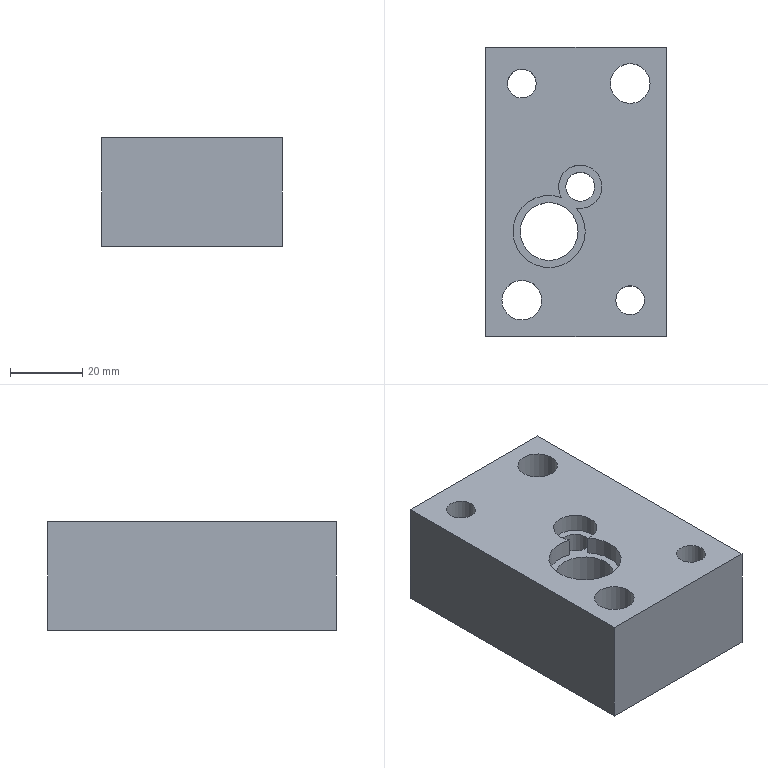Part | NX | features solid 2 | 1 solid | 19 faces | box 50 x 80 x 30 mm | volume 98920 mm3 | cylinder 10 | plane 9 | commonest cylinder face diameters 8 x3 11 x2 17 x2 12 x1 16 x1 20 x1
STEP:
#1=CARTESIAN_POINT('',(-537.829,181.45,124.));
#2=VERTEX_POINT('',#1);
#3=CARTESIAN_POINT('',(-533.829,181.45,124.));
#4=DIRECTION('',(0.,0.,-1.));
#5=DIRECTION('',(-1.,0.,0.));
#6=AXIS2_PLACEMENT_3D('',#3,#4,#5);
#7=CIRCLE('',#6,4.);
#8=EDGE_CURVE('',#2,#2,#7,.F.);
#9=ORIENTED_EDGE('',*,*,#8,.T.);
#10=EDGE_LOOP('',(#9));
#11=FACE_BOUND('',#10,.T.);
#12=CARTESIAN_POINT('',(-528.5,210.,124.));
#13=VERTEX_POINT('',#12);
#14=CARTESIAN_POINT('',(-520.,210.,124.));
#15=DIRECTION('',(0.,0.,-1.));
#16=DIRECTION('',(-1.,0.,0.));
#17=AXIS2_PLACEMENT_3D('',#14,#15,#16);
#18=CIRCLE('',#17,8.5);
#19=EDGE_CURVE('',#13,#13,#18,.T.);
#20=ORIENTED_EDGE('',*,*,#19,.F.);
#21=EDGE_LOOP('',(#20));
#22=FACE_BOUND('',#21,.T.);
#23=CARTESIAN_POINT('',(-558.5,150.,124.));
#24=VERTEX_POINT('',#23);
#25=CARTESIAN_POINT('',(-550.,150.,124.));
#26=DIRECTION('',(0.,0.,-1.));
#27=DIRECTION('',(-1.,0.,0.));
#28=AXIS2_PLACEMENT_3D('',#25,#26,#27);
#29=CIRCLE('',#28,8.5);
#30=EDGE_CURVE('',#24,#24,#29,.T.);
#31=ORIENTED_EDGE('',*,*,#30,.F.);
#32=EDGE_LOOP('',(#31));
#33=FACE_BOUND('',#32,.T.);
#34=CARTESIAN_POINT('',(-554.,210.,124.));
#35=VERTEX_POINT('',#34);
#36=CARTESIAN_POINT('',(-550.,210.,124.));
#37=DIRECTION('',(0.,0.,-1.));
#38=DIRECTION('',(-1.,0.,0.));
#39=AXIS2_PLACEMENT_3D('',#36,#37,#38);
#40=CIRCLE('',#39,4.);
#41=EDGE_CURVE('',#35,#35,#40,.T.);
#42=ORIENTED_EDGE('',*,*,#41,.F.);
#43=EDGE_LOOP('',(#42));
#44=FACE_BOUND('',#43,.T.);
#45=CARTESIAN_POINT('',(-524.,150.,124.));
#46=VERTEX_POINT('',#45);
#47=CARTESIAN_POINT('',(-520.,150.,124.));
#48=DIRECTION('',(0.,0.,-1.));
#49=DIRECTION('',(-1.,0.,0.));
#50=AXIS2_PLACEMENT_3D('',#47,#48,#49);
#51=CIRCLE('',#50,4.);
#52=EDGE_CURVE('',#46,#46,#51,.T.);
#53=ORIENTED_EDGE('',*,*,#52,.F.);
#54=EDGE_LOOP('',(#53));
#55=FACE_BOUND('',#54,.T.);
#56=CARTESIAN_POINT('',(-510.,220.,124.));
#57=VERTEX_POINT('',#56);
#58=CARTESIAN_POINT('',(-560.,220.,124.));
#59=VERTEX_POINT('',#58);
#60=CARTESIAN_POINT('',(-495.,220.,124.));
#61=DIRECTION('',(-1.,0.,0.));
#62=VECTOR('',#61,1000.);
#63=LINE('',#60,#62);
#64=EDGE_CURVE('',#57,#59,#63,.T.);
#65=ORIENTED_EDGE('',*,*,#64,.F.);
#66=CARTESIAN_POINT('',(-510.,140.,124.));
#67=VERTEX_POINT('',#66);
#68=CARTESIAN_POINT('',(-510.,205.,124.));
#69=DIRECTION('',(0.,1.,0.));
#70=VECTOR('',#69,1000.);
#71=LINE('',#68,#70);
#72=EDGE_CURVE('',#67,#57,#71,.T.);
#73=ORIENTED_EDGE('',*,*,#72,.F.);
#74=CARTESIAN_POINT('',(-560.,140.,124.));
#75=VERTEX_POINT('',#74);
#76=CARTESIAN_POINT('',(-495.,140.,124.));
#77=DIRECTION('',(1.,0.,0.));
#78=VECTOR('',#77,1000.);
#79=LINE('',#76,#78);
#80=EDGE_CURVE('',#75,#67,#79,.T.);
#81=ORIENTED_EDGE('',*,*,#80,.F.);
#82=CARTESIAN_POINT('',(-560.,205.,124.));
#83=DIRECTION('',(0.,-1.,0.));
#84=VECTOR('',#83,1000.);
#85=LINE('',#82,#84);
#86=EDGE_CURVE('',#59,#75,#85,.T.);
#87=ORIENTED_EDGE('',*,*,#86,.F.);
#88=EDGE_LOOP('',(#65,#73,#81,#87));
#89=FACE_BOUND('',#88,.T.);
#90=CARTESIAN_POINT('',(-550.438,169.049,124.));
#91=VERTEX_POINT('',#90);
#92=CARTESIAN_POINT('',(-542.438,169.049,124.));
#93=DIRECTION('',(0.,0.,-1.));
#94=DIRECTION('',(-1.,0.,0.));
#95=AXIS2_PLACEMENT_3D('',#92,#93,#94);
#96=CIRCLE('',#95,8.);
#97=EDGE_CURVE('',#91,#91,#96,.F.);
#98=ORIENTED_EDGE('',*,*,#97,.T.);
#99=EDGE_LOOP('',(#98));
#100=FACE_BOUND('',#99,.T.);
#101=CARTESIAN_POINT('',(-495.,205.,124.));
#102=DIRECTION('',(0.,0.,-1.));
#103=DIRECTION('',(1.,0.,0.));
#104=AXIS2_PLACEMENT_3D('',#101,#102,#103);
#105=PLANE('',#104);
#106=ADVANCED_FACE('',(#11,#22,#33,#44,#55,#89,#100),#105,.T.);
#107=CARTESIAN_POINT('',(-510.,140.,154.));
#108=VERTEX_POINT('',#107);
#109=CARTESIAN_POINT('',(-510.,220.,154.));
#110=VERTEX_POINT('',#109);
#111=CARTESIAN_POINT('',(-510.,169.049,154.));
#112=DIRECTION('',(0.,-1.,0.));
#113=VECTOR('',#112,1000.);
#114=LINE('',#111,#113);
#115=EDGE_CURVE('',#108,#110,#114,.F.);
#116=ORIENTED_EDGE('',*,*,#115,.F.);
#117=CARTESIAN_POINT('',(-510.,140.,128.));
#118=DIRECTION('',(0.,0.,1.));
#119=VECTOR('',#118,1000.);
#120=LINE('',#117,#119);
#121=EDGE_CURVE('',#67,#108,#120,.T.);
#122=ORIENTED_EDGE('',*,*,#121,.F.);
#123=ORIENTED_EDGE('',*,*,#72,.T.);
#124=CARTESIAN_POINT('',(-510.,220.,128.));
#125=DIRECTION('',(0.,0.,1.));
#126=VECTOR('',#125,1000.);
#127=LINE('',#124,#126);
#128=EDGE_CURVE('',#57,#110,#127,.T.);
#129=ORIENTED_EDGE('',*,*,#128,.T.);
#130=EDGE_LOOP('',(#116,#122,#123,#129));
#131=FACE_BOUND('',#130,.T.);
#132=CARTESIAN_POINT('',(-510.,155.,128.));
#133=DIRECTION('',(-1.,0.,0.));
#134=DIRECTION('',(0.,0.,-1.));
#135=AXIS2_PLACEMENT_3D('',#132,#133,#134);
#136=PLANE('',#135);
#137=ADVANCED_FACE('',(#131),#136,.F.);
#138=CARTESIAN_POINT('',(-560.,220.,154.));
#139=VERTEX_POINT('',#138);
#140=CARTESIAN_POINT('',(-542.438,220.,154.));
#141=DIRECTION('',(1.,0.,0.));
#142=VECTOR('',#141,1000.);
#143=LINE('',#140,#142);
#144=EDGE_CURVE('',#110,#139,#143,.F.);
#145=ORIENTED_EDGE('',*,*,#144,.F.);
#146=ORIENTED_EDGE('',*,*,#128,.F.);
#147=ORIENTED_EDGE('',*,*,#64,.T.);
#148=CARTESIAN_POINT('',(-560.,220.,128.));
#149=DIRECTION('',(0.,0.,1.));
#150=VECTOR('',#149,1000.);
#151=LINE('',#148,#150);
#152=EDGE_CURVE('',#59,#139,#151,.T.);
#153=ORIENTED_EDGE('',*,*,#152,.T.);
#154=EDGE_LOOP('',(#145,#146,#147,#153));
#155=FACE_BOUND('',#154,.T.);
#156=CARTESIAN_POINT('',(-495.,220.,128.));
#157=DIRECTION('',(0.,-1.,0.));
#158=DIRECTION('',(0.,0.,-1.));
#159=AXIS2_PLACEMENT_3D('',#156,#157,#158);
#160=PLANE('',#159);
#161=ADVANCED_FACE('',(#155),#160,.F.);
#162=ORIENTED_EDGE('',*,*,#86,.T.);
#163=CARTESIAN_POINT('',(-560.,140.,154.));
#164=VERTEX_POINT('',#163);
#165=CARTESIAN_POINT('',(-560.,140.,128.));
#166=DIRECTION('',(0.,0.,1.));
#167=VECTOR('',#166,1000.);
#168=LINE('',#165,#167);
#169=EDGE_CURVE('',#75,#164,#168,.T.);
#170=ORIENTED_EDGE('',*,*,#169,.T.);
#171=CARTESIAN_POINT('',(-560.,169.049,154.));
#172=DIRECTION('',(0.,1.,0.));
#173=VECTOR('',#172,1000.);
#174=LINE('',#171,#173);
#175=EDGE_CURVE('',#139,#164,#174,.F.);
#176=ORIENTED_EDGE('',*,*,#175,.F.);
#177=ORIENTED_EDGE('',*,*,#152,.F.);
#178=EDGE_LOOP('',(#162,#170,#176,#177));
#179=FACE_BOUND('',#178,.T.);
#180=CARTESIAN_POINT('',(-560.,205.,128.));
#181=DIRECTION('',(1.,0.,0.));
#182=DIRECTION('',(0.,0.,1.));
#183=AXIS2_PLACEMENT_3D('',#180,#181,#182);
#184=PLANE('',#183);
#185=ADVANCED_FACE('',(#179),#184,.F.);
#186=CARTESIAN_POINT('',(-542.438,140.,154.));
#187=DIRECTION('',(-1.,0.,0.));
#188=VECTOR('',#187,1000.);
#189=LINE('',#186,#188);
#190=EDGE_CURVE('',#164,#108,#189,.F.);
#191=ORIENTED_EDGE('',*,*,#190,.F.);
#192=ORIENTED_EDGE('',*,*,#169,.F.);
#193=ORIENTED_EDGE('',*,*,#80,.T.);
#194=ORIENTED_EDGE('',*,*,#121,.T.);
#195=EDGE_LOOP('',(#191,#192,#193,#194));
#196=FACE_BOUND('',#195,.T.);
#197=CARTESIAN_POINT('',(-550.,140.,128.));
#198=DIRECTION('',(0.,1.,0.));
#199=DIRECTION('',(0.,0.,1.));
#200=AXIS2_PLACEMENT_3D('',#197,#198,#199);
#201=PLANE('',#200);
#202=ADVANCED_FACE('',(#196),#201,.F.);
#203=CARTESIAN_POINT('',(-539.024,178.448,154.));
#204=VERTEX_POINT('',#203);
#205=CARTESIAN_POINT('',(-534.825,175.533,154.));
#206=VERTEX_POINT('',#205);
#207=CARTESIAN_POINT('',(-542.438,169.049,154.));
#208=DIRECTION('',(0.,0.,1.));
#209=DIRECTION('',(1.,0.,0.));
#210=AXIS2_PLACEMENT_3D('',#207,#208,#209);
#211=CIRCLE('',#210,10.);
#212=EDGE_CURVE('',#204,#206,#211,.T.);
#213=ORIENTED_EDGE('',*,*,#212,.F.);
#214=CARTESIAN_POINT('',(-533.829,181.45,154.));
#215=DIRECTION('',(0.,0.,1.));
#216=DIRECTION('',(1.,0.,0.));
#217=AXIS2_PLACEMENT_3D('',#214,#215,#216);
#218=CIRCLE('',#217,6.);
#219=EDGE_CURVE('',#206,#204,#218,.T.);
#220=ORIENTED_EDGE('',*,*,#219,.F.);
#221=EDGE_LOOP('',(#213,#220));
#222=FACE_BOUND('',#221,.T.);
#223=CARTESIAN_POINT('',(-514.5,210.,154.));
#224=VERTEX_POINT('',#223);
#225=CARTESIAN_POINT('',(-520.,210.,154.));
#226=DIRECTION('',(0.,0.,1.));
#227=DIRECTION('',(1.,0.,0.));
#228=AXIS2_PLACEMENT_3D('',#225,#226,#227);
#229=CIRCLE('',#228,5.5);
#230=EDGE_CURVE('',#224,#224,#229,.T.);
#231=ORIENTED_EDGE('',*,*,#230,.F.);
#232=EDGE_LOOP('',(#231));
#233=FACE_BOUND('',#232,.T.);
#234=CARTESIAN_POINT('',(-544.5,150.,154.));
#235=VERTEX_POINT('',#234);
#236=CARTESIAN_POINT('',(-550.,150.,154.));
#237=DIRECTION('',(0.,0.,1.));
#238=DIRECTION('',(1.,0.,0.));
#239=AXIS2_PLACEMENT_3D('',#236,#237,#238);
#240=CIRCLE('',#239,5.5);
#241=EDGE_CURVE('',#235,#235,#240,.T.);
#242=ORIENTED_EDGE('',*,*,#241,.F.);
#243=EDGE_LOOP('',(#242));
#244=FACE_BOUND('',#243,.T.);
#245=CARTESIAN_POINT('',(-546.,210.,154.));
#246=VERTEX_POINT('',#245);
#247=CARTESIAN_POINT('',(-550.,210.,154.));
#248=DIRECTION('',(0.,0.,1.));
#249=DIRECTION('',(1.,0.,0.));
#250=AXIS2_PLACEMENT_3D('',#247,#248,#249);
#251=CIRCLE('',#250,4.);
#252=EDGE_CURVE('',#246,#246,#251,.T.);
#253=ORIENTED_EDGE('',*,*,#252,.F.);
#254=EDGE_LOOP('',(#253));
#255=FACE_BOUND('',#254,.T.);
#256=CARTESIAN_POINT('',(-516.,150.,154.));
#257=VERTEX_POINT('',#256);
#258=CARTESIAN_POINT('',(-520.,150.,154.));
#259=DIRECTION('',(0.,0.,1.));
#260=DIRECTION('',(1.,0.,0.));
#261=AXIS2_PLACEMENT_3D('',#258,#259,#260);
#262=CIRCLE('',#261,4.);
#263=EDGE_CURVE('',#257,#257,#262,.T.);
#264=ORIENTED_EDGE('',*,*,#263,.F.);
#265=EDGE_LOOP('',(#264));
#266=FACE_BOUND('',#265,.T.);
#267=ORIENTED_EDGE('',*,*,#175,.T.);
#268=ORIENTED_EDGE('',*,*,#190,.T.);
#269=ORIENTED_EDGE('',*,*,#115,.T.);
#270=ORIENTED_EDGE('',*,*,#144,.T.);
#271=EDGE_LOOP('',(#267,#268,#269,#270));
#272=FACE_BOUND('',#271,.T.);
#273=CARTESIAN_POINT('',(-542.438,169.049,154.));
#274=DIRECTION('',(0.,0.,1.));
#275=DIRECTION('',(1.,0.,0.));
#276=AXIS2_PLACEMENT_3D('',#273,#274,#275);
#277=PLANE('',#276);
#278=ADVANCED_FACE('',(#222,#233,#244,#255,#266,#272),#277,.T.);
#279=ORIENTED_EDGE('',*,*,#263,.T.);
#280=EDGE_LOOP('',(#279));
#281=FACE_BOUND('',#280,.T.);
#282=ORIENTED_EDGE('',*,*,#52,.T.);
#283=EDGE_LOOP('',(#282));
#284=FACE_BOUND('',#283,.T.);
#285=CARTESIAN_POINT('',(-520.,150.,178.));
#286=DIRECTION('',(0.,0.,1.));
#287=DIRECTION('',(-1.,0.,0.));
#288=AXIS2_PLACEMENT_3D('',#285,#286,#287);
#289=CYLINDRICAL_SURFACE('',#288,4.);
#290=ADVANCED_FACE('',(#281,#284),#289,.F.);
#291=ORIENTED_EDGE('',*,*,#252,.T.);
#292=EDGE_LOOP('',(#291));
#293=FACE_BOUND('',#292,.T.);
#294=ORIENTED_EDGE('',*,*,#41,.T.);
#295=EDGE_LOOP('',(#294));
#296=FACE_BOUND('',#295,.T.);
#297=CARTESIAN_POINT('',(-550.,210.,178.));
#298=DIRECTION('',(0.,0.,1.));
#299=DIRECTION('',(-1.,0.,0.));
#300=AXIS2_PLACEMENT_3D('',#297,#298,#299);
#301=CYLINDRICAL_SURFACE('',#300,4.);
#302=ADVANCED_FACE('',(#293,#296),#301,.F.);
#303=CARTESIAN_POINT('',(-544.5,150.,139.));
#304=VERTEX_POINT('',#303);
#305=CARTESIAN_POINT('',(-550.,150.,139.));
#306=DIRECTION('',(0.,0.,1.));
#307=DIRECTION('',(1.,0.,0.));
#308=AXIS2_PLACEMENT_3D('',#305,#306,#307);
#309=CIRCLE('',#308,5.5);
#310=EDGE_CURVE('',#304,#304,#309,.F.);
#311=ORIENTED_EDGE('',*,*,#310,.T.);
#312=EDGE_LOOP('',(#311));
#313=FACE_BOUND('',#312,.T.);
#314=ORIENTED_EDGE('',*,*,#241,.T.);
#315=EDGE_LOOP('',(#314));
#316=FACE_BOUND('',#315,.T.);
#317=CARTESIAN_POINT('',(-550.,150.,178.));
#318=DIRECTION('',(0.,0.,1.));
#319=DIRECTION('',(-1.,0.,0.));
#320=AXIS2_PLACEMENT_3D('',#317,#318,#319);
#321=CYLINDRICAL_SURFACE('',#320,5.5);
#322=ADVANCED_FACE('',(#313,#316),#321,.F.);
#323=ORIENTED_EDGE('',*,*,#310,.F.);
#324=EDGE_LOOP('',(#323));
#325=FACE_BOUND('',#324,.T.);
#326=CARTESIAN_POINT('',(-541.5,150.,139.));
#327=VERTEX_POINT('',#326);
#328=CARTESIAN_POINT('',(-550.,150.,139.));
#329=DIRECTION('',(0.,0.,1.));
#330=DIRECTION('',(1.,0.,0.));
#331=AXIS2_PLACEMENT_3D('',#328,#329,#330);
#332=CIRCLE('',#331,8.5);
#333=EDGE_CURVE('',#327,#327,#332,.F.);
#334=ORIENTED_EDGE('',*,*,#333,.T.);
#335=EDGE_LOOP('',(#334));
#336=FACE_BOUND('',#335,.T.);
#337=CARTESIAN_POINT('',(-550.,150.,139.));
#338=DIRECTION('',(0.,0.,1.));
#339=DIRECTION('',(-1.,0.,0.));
#340=AXIS2_PLACEMENT_3D('',#337,#338,#339);
#341=PLANE('',#340);
#342=ADVANCED_FACE('',(#325,#336),#341,.F.);
#343=ORIENTED_EDGE('',*,*,#333,.F.);
#344=EDGE_LOOP('',(#343));
#345=FACE_BOUND('',#344,.T.);
#346=ORIENTED_EDGE('',*,*,#30,.T.);
#347=EDGE_LOOP('',(#346));
#348=FACE_BOUND('',#347,.T.);
#349=CARTESIAN_POINT('',(-550.,150.,128.));
#350=DIRECTION('',(0.,0.,1.));
#351=DIRECTION('',(-1.,0.,0.));
#352=AXIS2_PLACEMENT_3D('',#349,#350,#351);
#353=CYLINDRICAL_SURFACE('',#352,8.5);
#354=ADVANCED_FACE('',(#345,#348),#353,.F.);
#355=CARTESIAN_POINT('',(-514.5,210.,139.));
#356=VERTEX_POINT('',#355);
#357=CARTESIAN_POINT('',(-520.,210.,139.));
#358=DIRECTION('',(0.,0.,1.));
#359=DIRECTION('',(1.,0.,0.));
#360=AXIS2_PLACEMENT_3D('',#357,#358,#359);
#361=CIRCLE('',#360,5.5);
#362=EDGE_CURVE('',#356,#356,#361,.F.);
#363=ORIENTED_EDGE('',*,*,#362,.T.);
#364=EDGE_LOOP('',(#363));
#365=FACE_BOUND('',#364,.T.);
#366=ORIENTED_EDGE('',*,*,#230,.T.);
#367=EDGE_LOOP('',(#366));
#368=FACE_BOUND('',#367,.T.);
#369=CARTESIAN_POINT('',(-520.,210.,178.));
#370=DIRECTION('',(0.,0.,1.));
#371=DIRECTION('',(-1.,0.,0.));
#372=AXIS2_PLACEMENT_3D('',#369,#370,#371);
#373=CYLINDRICAL_SURFACE('',#372,5.5);
#374=ADVANCED_FACE('',(#365,#368),#373,.F.);
#375=ORIENTED_EDGE('',*,*,#362,.F.);
#376=EDGE_LOOP('',(#375));
#377=FACE_BOUND('',#376,.T.);
#378=CARTESIAN_POINT('',(-511.5,210.,139.));
#379=VERTEX_POINT('',#378);
#380=CARTESIAN_POINT('',(-520.,210.,139.));
#381=DIRECTION('',(0.,0.,1.));
#382=DIRECTION('',(1.,0.,0.));
#383=AXIS2_PLACEMENT_3D('',#380,#381,#382);
#384=CIRCLE('',#383,8.5);
#385=EDGE_CURVE('',#379,#379,#384,.F.);
#386=ORIENTED_EDGE('',*,*,#385,.T.);
#387=EDGE_LOOP('',(#386));
#388=FACE_BOUND('',#387,.T.);
#389=CARTESIAN_POINT('',(-520.,210.,139.));
#390=DIRECTION('',(0.,0.,1.));
#391=DIRECTION('',(-1.,0.,0.));
#392=AXIS2_PLACEMENT_3D('',#389,#390,#391);
#393=PLANE('',#392);
#394=ADVANCED_FACE('',(#377,#388),#393,.F.);
#395=ORIENTED_EDGE('',*,*,#385,.F.);
#396=EDGE_LOOP('',(#395));
#397=FACE_BOUND('',#396,.T.);
#398=ORIENTED_EDGE('',*,*,#19,.T.);
#399=EDGE_LOOP('',(#398));
#400=FACE_BOUND('',#399,.T.);
#401=CARTESIAN_POINT('',(-520.,210.,128.));
#402=DIRECTION('',(0.,0.,1.));
#403=DIRECTION('',(-1.,0.,0.));
#404=AXIS2_PLACEMENT_3D('',#401,#402,#403);
#405=CYLINDRICAL_SURFACE('',#404,8.5);
#406=ADVANCED_FACE('',(#397,#400),#405,.F.);
#407=ORIENTED_EDGE('',*,*,#8,.F.);
#408=EDGE_LOOP('',(#407));
#409=FACE_BOUND('',#408,.T.);
#410=CARTESIAN_POINT('',(-529.829,181.45,149.));
#411=VERTEX_POINT('',#410);
#412=CARTESIAN_POINT('',(-533.829,181.45,149.));
#413=DIRECTION('',(0.,0.,1.));
#414=DIRECTION('',(1.,0.,0.));
#415=AXIS2_PLACEMENT_3D('',#412,#413,#414);
#416=CIRCLE('',#415,4.);
#417=EDGE_CURVE('',#411,#411,#416,.T.);
#418=ORIENTED_EDGE('',*,*,#417,.T.);
#419=EDGE_LOOP('',(#418));
#420=FACE_BOUND('',#419,.T.);
#421=CARTESIAN_POINT('',(-533.829,181.45,154.));
#422=DIRECTION('',(0.,0.,-1.));
#423=DIRECTION('',(-1.,0.,0.));
#424=AXIS2_PLACEMENT_3D('',#421,#422,#423);
#425=CYLINDRICAL_SURFACE('',#424,4.);
#426=ADVANCED_FACE('',(#409,#420),#425,.F.);
#427=CARTESIAN_POINT('',(-534.825,175.533,149.));
#428=VERTEX_POINT('',#427);
#429=CARTESIAN_POINT('',(-539.024,178.448,149.));
#430=VERTEX_POINT('',#429);
#431=CARTESIAN_POINT('',(-533.829,181.45,149.));
#432=DIRECTION('',(0.,0.,1.));
#433=DIRECTION('',(1.,0.,0.));
#434=AXIS2_PLACEMENT_3D('',#431,#432,#433);
#435=CIRCLE('',#434,6.);
#436=EDGE_CURVE('',#428,#430,#435,.T.);
#437=ORIENTED_EDGE('',*,*,#436,.T.);
#438=CARTESIAN_POINT('',(-542.438,169.049,149.));
#439=DIRECTION('',(0.,0.,1.));
#440=DIRECTION('',(1.,0.,0.));
#441=AXIS2_PLACEMENT_3D('',#438,#439,#440);
#442=CIRCLE('',#441,10.);
#443=EDGE_CURVE('',#430,#428,#442,.T.);
#444=ORIENTED_EDGE('',*,*,#443,.T.);
#445=EDGE_LOOP('',(#437,#444));
#446=FACE_BOUND('',#445,.T.);
#447=ORIENTED_EDGE('',*,*,#417,.F.);
#448=EDGE_LOOP('',(#447));
#449=FACE_BOUND('',#448,.T.);
#450=CARTESIAN_POINT('',(-534.438,169.049,149.));
#451=VERTEX_POINT('',#450);
#452=CARTESIAN_POINT('',(-542.438,169.049,149.));
#453=DIRECTION('',(0.,0.,1.));
#454=DIRECTION('',(1.,0.,0.));
#455=AXIS2_PLACEMENT_3D('',#452,#453,#454);
#456=CIRCLE('',#455,8.);
#457=EDGE_CURVE('',#451,#451,#456,.T.);
#458=ORIENTED_EDGE('',*,*,#457,.F.);
#459=EDGE_LOOP('',(#458));
#460=FACE_BOUND('',#459,.T.);
#461=CARTESIAN_POINT('',(-533.829,181.45,149.));
#462=DIRECTION('',(0.,0.,1.));
#463=DIRECTION('',(1.,0.,0.));
#464=AXIS2_PLACEMENT_3D('',#461,#462,#463);
#465=PLANE('',#464);
#466=ADVANCED_FACE('',(#446,#449,#460),#465,.T.);
#467=CARTESIAN_POINT('',(-534.825,175.533,149.));
#468=DIRECTION('',(0.,0.,-1.));
#469=VECTOR('',#468,1000.);
#470=LINE('',#467,#469);
#471=EDGE_CURVE('',#206,#428,#470,.T.);
#472=ORIENTED_EDGE('',*,*,#471,.F.);
#473=ORIENTED_EDGE('',*,*,#219,.T.);
#474=CARTESIAN_POINT('',(-539.024,178.448,149.));
#475=DIRECTION('',(0.,0.,-1.));
#476=VECTOR('',#475,1000.);
#477=LINE('',#474,#476);
#478=EDGE_CURVE('',#430,#204,#477,.F.);
#479=ORIENTED_EDGE('',*,*,#478,.F.);
#480=ORIENTED_EDGE('',*,*,#436,.F.);
#481=EDGE_LOOP('',(#472,#473,#479,#480));
#482=FACE_BOUND('',#481,.T.);
#483=CARTESIAN_POINT('',(-533.829,181.45,149.));
#484=DIRECTION('',(0.,0.,1.));
#485=DIRECTION('',(1.,0.,0.));
#486=AXIS2_PLACEMENT_3D('',#483,#484,#485);
#487=CYLINDRICAL_SURFACE('',#486,6.);
#488=ADVANCED_FACE('',(#482),#487,.F.);
#489=ORIENTED_EDGE('',*,*,#97,.F.);
#490=EDGE_LOOP('',(#489));
#491=FACE_BOUND('',#490,.T.);
#492=ORIENTED_EDGE('',*,*,#457,.T.);
#493=EDGE_LOOP('',(#492));
#494=FACE_BOUND('',#493,.T.);
#495=CARTESIAN_POINT('',(-542.438,169.049,154.));
#496=DIRECTION('',(0.,0.,-1.));
#497=DIRECTION('',(-1.,0.,0.));
#498=AXIS2_PLACEMENT_3D('',#495,#496,#497);
#499=CYLINDRICAL_SURFACE('',#498,8.);
#500=ADVANCED_FACE('',(#491,#494),#499,.F.);
#501=ORIENTED_EDGE('',*,*,#212,.T.);
#502=ORIENTED_EDGE('',*,*,#471,.T.);
#503=ORIENTED_EDGE('',*,*,#443,.F.);
#504=ORIENTED_EDGE('',*,*,#478,.T.);
#505=EDGE_LOOP('',(#501,#502,#503,#504));
#506=FACE_BOUND('',#505,.T.);
#507=CARTESIAN_POINT('',(-542.438,169.049,149.));
#508=DIRECTION('',(0.,0.,1.));
#509=DIRECTION('',(1.,0.,0.));
#510=AXIS2_PLACEMENT_3D('',#507,#508,#509);
#511=CYLINDRICAL_SURFACE('',#510,10.);
#512=ADVANCED_FACE('',(#506),#511,.F.);
#513=CLOSED_SHELL('',(#106,#137,#161,#185,#202,#278,#290,#302,#322,#342,#354,#374,#394,#406,#426,#466,#488,#500,#512));
#514=MANIFOLD_SOLID_BREP('',#513);
#515=(LENGTH_UNIT()NAMED_UNIT(*)SI_UNIT(.MILLI.,.METRE.));
#516=UNCERTAINTY_MEASURE_WITH_UNIT(LENGTH_MEASURE(0.00001),#515,'','');
#517=(NAMED_UNIT(*)PLANE_ANGLE_UNIT()SI_UNIT($,.RADIAN.));
#518=(NAMED_UNIT(*)SI_UNIT($,.STERADIAN.)SOLID_ANGLE_UNIT());
#519=(GEOMETRIC_REPRESENTATION_CONTEXT(3)GLOBAL_UNCERTAINTY_ASSIGNED_CONTEXT((#516))GLOBAL_UNIT_ASSIGNED_CONTEXT((#515,#517,#518))REPRESENTATION_CONTEXT('',''));
#520=ADVANCED_BREP_SHAPE_REPRESENTATION('',(#514),#519);